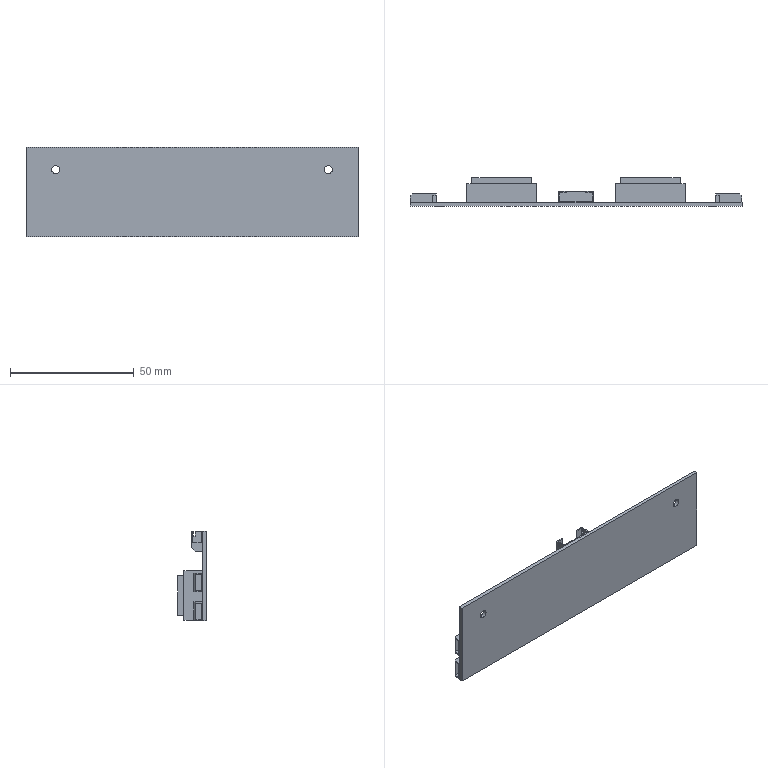Part | SolidWorks | features BaseBody 1 | 1 solid | 125 faces | box 134 x 11.5 x 36 mm | volume 18226 mm3 | plane 121 | cylinder 4 | commonest cylinder face diameters 3.25 x4